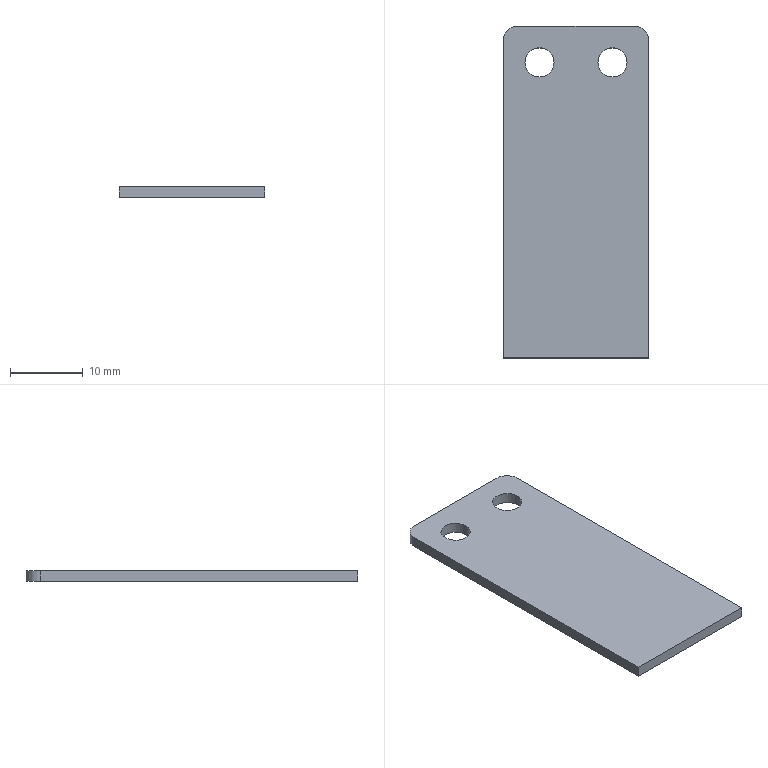Part | NX | 1 solid | 10 faces | box 20 x 45.5 x 1.5 mm | volume 1325 mm3 | plane 6 | cylinder 4 | commonest cylinder face diameters 4 x4
STEP:
#1=CARTESIAN_POINT('',(-10.,20.75,0.));
#2=VERTEX_POINT('',#1);
#3=CARTESIAN_POINT('',(-10.,-22.75,0.));
#4=VERTEX_POINT('',#3);
#5=CARTESIAN_POINT('',(-10.,22.75,0.));
#6=DIRECTION('',(0.,-1.,0.));
#7=VECTOR('',#6,1000.);
#8=LINE('',#5,#7);
#9=EDGE_CURVE('',#2,#4,#8,.T.);
#10=ORIENTED_EDGE('',*,*,#9,.F.);
#11=CARTESIAN_POINT('',(-10.,20.75,-1.5));
#12=VERTEX_POINT('',#11);
#13=CARTESIAN_POINT('',(-10.,20.75,-1.5));
#14=DIRECTION('',(0.,0.,1.));
#15=VECTOR('',#14,1000.);
#16=LINE('',#13,#15);
#17=EDGE_CURVE('',#2,#12,#16,.F.);
#18=ORIENTED_EDGE('',*,*,#17,.T.);
#19=CARTESIAN_POINT('',(-10.,-22.75,-1.5));
#20=VERTEX_POINT('',#19);
#21=CARTESIAN_POINT('',(-10.,22.75,-1.5));
#22=DIRECTION('',(0.,-1.,0.));
#23=VECTOR('',#22,1000.);
#24=LINE('',#21,#23);
#25=EDGE_CURVE('',#12,#20,#24,.T.);
#26=ORIENTED_EDGE('',*,*,#25,.T.);
#27=CARTESIAN_POINT('',(-10.,-22.75,-1.5));
#28=DIRECTION('',(0.,0.,1.));
#29=VECTOR('',#28,1000.);
#30=LINE('',#27,#29);
#31=EDGE_CURVE('',#20,#4,#30,.T.);
#32=ORIENTED_EDGE('',*,*,#31,.T.);
#33=EDGE_LOOP('',(#10,#18,#26,#32));
#34=FACE_BOUND('',#33,.T.);
#35=CARTESIAN_POINT('',(-10.,22.75,-1.5));
#36=DIRECTION('',(-1.,0.,0.));
#37=DIRECTION('',(0.,-1.,0.));
#38=AXIS2_PLACEMENT_3D('',#35,#36,#37);
#39=PLANE('',#38);
#40=ADVANCED_FACE('',(#34),#39,.T.);
#41=CARTESIAN_POINT('',(8.,22.75,0.));
#42=VERTEX_POINT('',#41);
#43=CARTESIAN_POINT('',(-8.,22.75,0.));
#44=VERTEX_POINT('',#43);
#45=CARTESIAN_POINT('',(10.,22.75,0.));
#46=DIRECTION('',(-1.,0.,0.));
#47=VECTOR('',#46,1000.);
#48=LINE('',#45,#47);
#49=EDGE_CURVE('',#42,#44,#48,.T.);
#50=ORIENTED_EDGE('',*,*,#49,.F.);
#51=CARTESIAN_POINT('',(8.,22.75,-1.5));
#52=VERTEX_POINT('',#51);
#53=CARTESIAN_POINT('',(8.,22.75,-1.5));
#54=DIRECTION('',(0.,0.,1.));
#55=VECTOR('',#54,1000.);
#56=LINE('',#53,#55);
#57=EDGE_CURVE('',#42,#52,#56,.F.);
#58=ORIENTED_EDGE('',*,*,#57,.T.);
#59=CARTESIAN_POINT('',(-8.,22.75,-1.5));
#60=VERTEX_POINT('',#59);
#61=CARTESIAN_POINT('',(10.,22.75,-1.5));
#62=DIRECTION('',(-1.,0.,0.));
#63=VECTOR('',#62,1000.);
#64=LINE('',#61,#63);
#65=EDGE_CURVE('',#52,#60,#64,.T.);
#66=ORIENTED_EDGE('',*,*,#65,.T.);
#67=CARTESIAN_POINT('',(-8.,22.75,-1.5));
#68=DIRECTION('',(0.,0.,1.));
#69=VECTOR('',#68,1000.);
#70=LINE('',#67,#69);
#71=EDGE_CURVE('',#60,#44,#70,.T.);
#72=ORIENTED_EDGE('',*,*,#71,.T.);
#73=EDGE_LOOP('',(#50,#58,#66,#72));
#74=FACE_BOUND('',#73,.T.);
#75=CARTESIAN_POINT('',(10.,22.75,-1.5));
#76=DIRECTION('',(0.,1.,0.));
#77=DIRECTION('',(0.,0.,1.));
#78=AXIS2_PLACEMENT_3D('',#75,#76,#77);
#79=PLANE('',#78);
#80=ADVANCED_FACE('',(#74),#79,.T.);
#81=CARTESIAN_POINT('',(10.,-22.75,-1.5));
#82=VERTEX_POINT('',#81);
#83=CARTESIAN_POINT('',(10.,20.75,-1.5));
#84=VERTEX_POINT('',#83);
#85=CARTESIAN_POINT('',(10.,22.75,-1.5));
#86=DIRECTION('',(0.,1.,0.));
#87=VECTOR('',#86,1000.);
#88=LINE('',#85,#87);
#89=EDGE_CURVE('',#82,#84,#88,.T.);
#90=ORIENTED_EDGE('',*,*,#89,.T.);
#91=CARTESIAN_POINT('',(10.,20.75,0.));
#92=VERTEX_POINT('',#91);
#93=CARTESIAN_POINT('',(10.,20.75,-1.5));
#94=DIRECTION('',(0.,0.,1.));
#95=VECTOR('',#94,1000.);
#96=LINE('',#93,#95);
#97=EDGE_CURVE('',#84,#92,#96,.T.);
#98=ORIENTED_EDGE('',*,*,#97,.T.);
#99=CARTESIAN_POINT('',(10.,-22.75,0.));
#100=VERTEX_POINT('',#99);
#101=CARTESIAN_POINT('',(10.,22.75,0.));
#102=DIRECTION('',(0.,1.,0.));
#103=VECTOR('',#102,1000.);
#104=LINE('',#101,#103);
#105=EDGE_CURVE('',#100,#92,#104,.T.);
#106=ORIENTED_EDGE('',*,*,#105,.F.);
#107=CARTESIAN_POINT('',(10.,-22.75,-1.5));
#108=DIRECTION('',(0.,0.,1.));
#109=VECTOR('',#108,1000.);
#110=LINE('',#107,#109);
#111=EDGE_CURVE('',#82,#100,#110,.T.);
#112=ORIENTED_EDGE('',*,*,#111,.F.);
#113=EDGE_LOOP('',(#90,#98,#106,#112));
#114=FACE_BOUND('',#113,.T.);
#115=CARTESIAN_POINT('',(10.,22.75,-1.5));
#116=DIRECTION('',(1.,0.,0.));
#117=DIRECTION('',(0.,1.,0.));
#118=AXIS2_PLACEMENT_3D('',#115,#116,#117);
#119=PLANE('',#118);
#120=ADVANCED_FACE('',(#114),#119,.T.);
#121=CARTESIAN_POINT('',(10.,-22.75,0.));
#122=DIRECTION('',(1.,0.,0.));
#123=VECTOR('',#122,1000.);
#124=LINE('',#121,#123);
#125=EDGE_CURVE('',#4,#100,#124,.T.);
#126=ORIENTED_EDGE('',*,*,#125,.F.);
#127=ORIENTED_EDGE('',*,*,#31,.F.);
#128=CARTESIAN_POINT('',(10.,-22.75,-1.5));
#129=DIRECTION('',(1.,0.,0.));
#130=VECTOR('',#129,1000.);
#131=LINE('',#128,#130);
#132=EDGE_CURVE('',#20,#82,#131,.T.);
#133=ORIENTED_EDGE('',*,*,#132,.T.);
#134=ORIENTED_EDGE('',*,*,#111,.T.);
#135=EDGE_LOOP('',(#126,#127,#133,#134));
#136=FACE_BOUND('',#135,.T.);
#137=CARTESIAN_POINT('',(10.,-22.75,-1.5));
#138=DIRECTION('',(0.,-1.,0.));
#139=DIRECTION('',(0.,0.,-1.));
#140=AXIS2_PLACEMENT_3D('',#137,#138,#139);
#141=PLANE('',#140);
#142=ADVANCED_FACE('',(#136),#141,.T.);
#143=CARTESIAN_POINT('',(3.,17.75,-1.5));
#144=VERTEX_POINT('',#143);
#145=CARTESIAN_POINT('',(5.,17.75,-1.5));
#146=DIRECTION('',(0.,0.,1.));
#147=DIRECTION('',(-1.,0.,0.));
#148=AXIS2_PLACEMENT_3D('',#145,#146,#147);
#149=CIRCLE('',#148,2.);
#150=EDGE_CURVE('',#144,#144,#149,.T.);
#151=ORIENTED_EDGE('',*,*,#150,.T.);
#152=EDGE_LOOP('',(#151));
#153=FACE_BOUND('',#152,.T.);
#154=CARTESIAN_POINT('',(-3.,17.75,-1.5));
#155=VERTEX_POINT('',#154);
#156=CARTESIAN_POINT('',(-5.,17.75,-1.5));
#157=DIRECTION('',(0.,0.,1.));
#158=DIRECTION('',(1.,0.,0.));
#159=AXIS2_PLACEMENT_3D('',#156,#157,#158);
#160=CIRCLE('',#159,2.);
#161=EDGE_CURVE('',#155,#155,#160,.T.);
#162=ORIENTED_EDGE('',*,*,#161,.T.);
#163=EDGE_LOOP('',(#162));
#164=FACE_BOUND('',#163,.T.);
#165=ORIENTED_EDGE('',*,*,#65,.F.);
#166=CARTESIAN_POINT('',(8.,20.75,-1.5));
#167=DIRECTION('',(0.,0.,-1.));
#168=DIRECTION('',(-1.,0.,0.));
#169=AXIS2_PLACEMENT_3D('',#166,#167,#168);
#170=CIRCLE('',#169,2.);
#171=EDGE_CURVE('',#52,#84,#170,.T.);
#172=ORIENTED_EDGE('',*,*,#171,.T.);
#173=ORIENTED_EDGE('',*,*,#89,.F.);
#174=ORIENTED_EDGE('',*,*,#132,.F.);
#175=ORIENTED_EDGE('',*,*,#25,.F.);
#176=CARTESIAN_POINT('',(-8.,20.75,-1.5));
#177=DIRECTION('',(0.,0.,-1.));
#178=DIRECTION('',(-1.,0.,0.));
#179=AXIS2_PLACEMENT_3D('',#176,#177,#178);
#180=CIRCLE('',#179,2.);
#181=EDGE_CURVE('',#12,#60,#180,.T.);
#182=ORIENTED_EDGE('',*,*,#181,.T.);
#183=EDGE_LOOP('',(#165,#172,#173,#174,#175,#182));
#184=FACE_BOUND('',#183,.T.);
#185=CARTESIAN_POINT('',(0.,0.,-1.5));
#186=DIRECTION('',(0.,0.,-1.));
#187=DIRECTION('',(-1.,0.,0.));
#188=AXIS2_PLACEMENT_3D('',#185,#186,#187);
#189=PLANE('',#188);
#190=ADVANCED_FACE('',(#153,#164,#184),#189,.T.);
#191=CARTESIAN_POINT('',(3.,17.75,0.));
#192=VERTEX_POINT('',#191);
#193=CARTESIAN_POINT('',(5.,17.75,0.));
#194=DIRECTION('',(0.,0.,1.));
#195=DIRECTION('',(-1.,0.,0.));
#196=AXIS2_PLACEMENT_3D('',#193,#194,#195);
#197=CIRCLE('',#196,2.);
#198=EDGE_CURVE('',#192,#192,#197,.T.);
#199=ORIENTED_EDGE('',*,*,#198,.F.);
#200=EDGE_LOOP('',(#199));
#201=FACE_BOUND('',#200,.T.);
#202=CARTESIAN_POINT('',(-3.,17.75,0.));
#203=VERTEX_POINT('',#202);
#204=CARTESIAN_POINT('',(-5.,17.75,0.));
#205=DIRECTION('',(0.,0.,1.));
#206=DIRECTION('',(1.,0.,0.));
#207=AXIS2_PLACEMENT_3D('',#204,#205,#206);
#208=CIRCLE('',#207,2.);
#209=EDGE_CURVE('',#203,#203,#208,.T.);
#210=ORIENTED_EDGE('',*,*,#209,.F.);
#211=EDGE_LOOP('',(#210));
#212=FACE_BOUND('',#211,.T.);
#213=ORIENTED_EDGE('',*,*,#105,.T.);
#214=CARTESIAN_POINT('',(8.,20.75,0.));
#215=DIRECTION('',(0.,0.,-1.));
#216=DIRECTION('',(-1.,0.,0.));
#217=AXIS2_PLACEMENT_3D('',#214,#215,#216);
#218=CIRCLE('',#217,2.);
#219=EDGE_CURVE('',#92,#42,#218,.F.);
#220=ORIENTED_EDGE('',*,*,#219,.T.);
#221=ORIENTED_EDGE('',*,*,#49,.T.);
#222=CARTESIAN_POINT('',(-8.,20.75,0.));
#223=DIRECTION('',(0.,0.,-1.));
#224=DIRECTION('',(-1.,0.,0.));
#225=AXIS2_PLACEMENT_3D('',#222,#223,#224);
#226=CIRCLE('',#225,2.);
#227=EDGE_CURVE('',#44,#2,#226,.F.);
#228=ORIENTED_EDGE('',*,*,#227,.T.);
#229=ORIENTED_EDGE('',*,*,#9,.T.);
#230=ORIENTED_EDGE('',*,*,#125,.T.);
#231=EDGE_LOOP('',(#213,#220,#221,#228,#229,#230));
#232=FACE_BOUND('',#231,.T.);
#233=CARTESIAN_POINT('',(0.,0.,0.));
#234=DIRECTION('',(0.,0.,-1.));
#235=DIRECTION('',(-1.,0.,0.));
#236=AXIS2_PLACEMENT_3D('',#233,#234,#235);
#237=PLANE('',#236);
#238=ADVANCED_FACE('',(#201,#212,#232),#237,.F.);
#239=ORIENTED_EDGE('',*,*,#161,.F.);
#240=EDGE_LOOP('',(#239));
#241=FACE_BOUND('',#240,.T.);
#242=ORIENTED_EDGE('',*,*,#209,.T.);
#243=EDGE_LOOP('',(#242));
#244=FACE_BOUND('',#243,.T.);
#245=CARTESIAN_POINT('',(-5.,17.75,-1.5));
#246=DIRECTION('',(0.,0.,1.));
#247=DIRECTION('',(1.,0.,0.));
#248=AXIS2_PLACEMENT_3D('',#245,#246,#247);
#249=CYLINDRICAL_SURFACE('',#248,2.);
#250=ADVANCED_FACE('',(#241,#244),#249,.F.);
#251=ORIENTED_EDGE('',*,*,#150,.F.);
#252=EDGE_LOOP('',(#251));
#253=FACE_BOUND('',#252,.T.);
#254=ORIENTED_EDGE('',*,*,#198,.T.);
#255=EDGE_LOOP('',(#254));
#256=FACE_BOUND('',#255,.T.);
#257=CARTESIAN_POINT('',(5.,17.75,-1.5));
#258=DIRECTION('',(0.,0.,1.));
#259=DIRECTION('',(1.,0.,0.));
#260=AXIS2_PLACEMENT_3D('',#257,#258,#259);
#261=CYLINDRICAL_SURFACE('',#260,2.);
#262=ADVANCED_FACE('',(#253,#256),#261,.F.);
#263=ORIENTED_EDGE('',*,*,#171,.F.);
#264=ORIENTED_EDGE('',*,*,#57,.F.);
#265=ORIENTED_EDGE('',*,*,#219,.F.);
#266=ORIENTED_EDGE('',*,*,#97,.F.);
#267=EDGE_LOOP('',(#263,#264,#265,#266));
#268=FACE_BOUND('',#267,.T.);
#269=CARTESIAN_POINT('',(8.,20.75,-1.5));
#270=DIRECTION('',(0.,0.,1.));
#271=DIRECTION('',(1.,0.,0.));
#272=AXIS2_PLACEMENT_3D('',#269,#270,#271);
#273=CYLINDRICAL_SURFACE('',#272,2.);
#274=ADVANCED_FACE('',(#268),#273,.T.);
#275=ORIENTED_EDGE('',*,*,#181,.F.);
#276=ORIENTED_EDGE('',*,*,#17,.F.);
#277=ORIENTED_EDGE('',*,*,#227,.F.);
#278=ORIENTED_EDGE('',*,*,#71,.F.);
#279=EDGE_LOOP('',(#275,#276,#277,#278));
#280=FACE_BOUND('',#279,.T.);
#281=CARTESIAN_POINT('',(-8.,20.75,-1.5));
#282=DIRECTION('',(0.,0.,1.));
#283=DIRECTION('',(1.,0.,0.));
#284=AXIS2_PLACEMENT_3D('',#281,#282,#283);
#285=CYLINDRICAL_SURFACE('',#284,2.);
#286=ADVANCED_FACE('',(#280),#285,.T.);
#287=CLOSED_SHELL('',(#40,#80,#120,#142,#190,#238,#250,#262,#274,#286));
#288=MANIFOLD_SOLID_BREP('',#287);
#289=(LENGTH_UNIT()NAMED_UNIT(*)SI_UNIT(.MILLI.,.METRE.));
#290=UNCERTAINTY_MEASURE_WITH_UNIT(LENGTH_MEASURE(0.00001),#289,'','');
#291=(NAMED_UNIT(*)PLANE_ANGLE_UNIT()SI_UNIT($,.RADIAN.));
#292=(NAMED_UNIT(*)SI_UNIT($,.STERADIAN.)SOLID_ANGLE_UNIT());
#293=(GEOMETRIC_REPRESENTATION_CONTEXT(3)GLOBAL_UNCERTAINTY_ASSIGNED_CONTEXT((#290))GLOBAL_UNIT_ASSIGNED_CONTEXT((#289,#291,#292))REPRESENTATION_CONTEXT('',''));
#294=ADVANCED_BREP_SHAPE_REPRESENTATION('',(#288),#293);